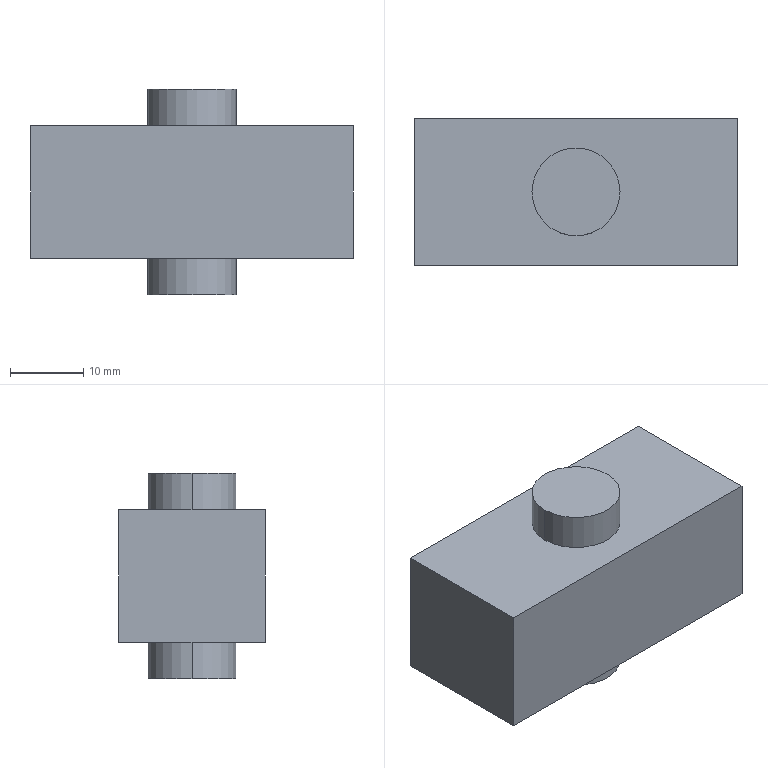Part | SolidWorks | features Extrusion 1, ICE 1 | 1 solid | 12 faces | box 44 x 20 x 28 mm | volume 16971 mm3 | plane 8 | cylinder 4 | commonest cylinder face diameters 12 x4
STEP:
#1=CARTESIAN_POINT('',(6.,0.,-14.));
#2=VERTEX_POINT('',#1);
#3=CARTESIAN_POINT('',(-6.,0.,-14.));
#4=VERTEX_POINT('',#3);
#5=CARTESIAN_POINT('',(0.,0.,-14.));
#6=DIRECTION('',(0.,0.,1.));
#7=DIRECTION('',(1.,0.,0.));
#8=AXIS2_PLACEMENT_3D('',#5,#6,#7);
#9=CIRCLE('',#8,6.);
#10=EDGE_CURVE('',#2,#4,#9,.T.);
#11=ORIENTED_EDGE('',*,*,#10,.T.);
#12=CARTESIAN_POINT('',(-6.,0.,-9.));
#13=VERTEX_POINT('',#12);
#14=CARTESIAN_POINT('',(-6.,0.,-14.));
#15=DIRECTION('',(0.,0.,1.));
#16=VECTOR('',#15,1000.);
#17=LINE('',#14,#16);
#18=EDGE_CURVE('',#4,#13,#17,.T.);
#19=ORIENTED_EDGE('',*,*,#18,.T.);
#20=CARTESIAN_POINT('',(6.,0.,-9.));
#21=VERTEX_POINT('',#20);
#22=CARTESIAN_POINT('',(0.,0.,-9.));
#23=DIRECTION('',(0.,0.,1.));
#24=DIRECTION('',(1.,0.,0.));
#25=AXIS2_PLACEMENT_3D('',#22,#23,#24);
#26=CIRCLE('',#25,6.);
#27=EDGE_CURVE('',#21,#13,#26,.T.);
#28=ORIENTED_EDGE('',*,*,#27,.F.);
#29=CARTESIAN_POINT('',(6.,0.,-14.));
#30=DIRECTION('',(0.,0.,1.));
#31=VECTOR('',#30,1000.);
#32=LINE('',#29,#31);
#33=EDGE_CURVE('',#2,#21,#32,.T.);
#34=ORIENTED_EDGE('',*,*,#33,.F.);
#35=EDGE_LOOP('',(#11,#19,#28,#34));
#36=FACE_OUTER_BOUND('',#35,.T.);
#37=CARTESIAN_POINT('',(0.,0.,-14.));
#38=DIRECTION('',(0.,0.,1.));
#39=DIRECTION('',(1.,0.,0.));
#40=AXIS2_PLACEMENT_3D('',#37,#38,#39);
#41=CYLINDRICAL_SURFACE('',#40,6.);
#42=ADVANCED_FACE('',(#36),#41,.T.);
#43=CARTESIAN_POINT('',(6.,0.,9.));
#44=VERTEX_POINT('',#43);
#45=CARTESIAN_POINT('',(-6.,0.,9.));
#46=VERTEX_POINT('',#45);
#47=CARTESIAN_POINT('',(0.,0.,9.));
#48=DIRECTION('',(0.,0.,1.));
#49=DIRECTION('',(1.,0.,0.));
#50=AXIS2_PLACEMENT_3D('',#47,#48,#49);
#51=CIRCLE('',#50,6.);
#52=EDGE_CURVE('',#44,#46,#51,.T.);
#53=ORIENTED_EDGE('',*,*,#52,.T.);
#54=CARTESIAN_POINT('',(-6.,0.,14.));
#55=VERTEX_POINT('',#54);
#56=CARTESIAN_POINT('',(-6.,0.,-14.));
#57=DIRECTION('',(0.,0.,1.));
#58=VECTOR('',#57,1000.);
#59=LINE('',#56,#58);
#60=EDGE_CURVE('',#46,#55,#59,.T.);
#61=ORIENTED_EDGE('',*,*,#60,.T.);
#62=CARTESIAN_POINT('',(6.,0.,14.));
#63=VERTEX_POINT('',#62);
#64=CARTESIAN_POINT('',(0.,0.,14.));
#65=DIRECTION('',(0.,0.,1.));
#66=DIRECTION('',(1.,0.,0.));
#67=AXIS2_PLACEMENT_3D('',#64,#65,#66);
#68=CIRCLE('',#67,6.);
#69=EDGE_CURVE('',#63,#55,#68,.T.);
#70=ORIENTED_EDGE('',*,*,#69,.F.);
#71=CARTESIAN_POINT('',(6.,0.,-14.));
#72=DIRECTION('',(0.,0.,1.));
#73=VECTOR('',#72,1000.);
#74=LINE('',#71,#73);
#75=EDGE_CURVE('',#44,#63,#74,.T.);
#76=ORIENTED_EDGE('',*,*,#75,.F.);
#77=EDGE_LOOP('',(#53,#61,#70,#76));
#78=FACE_OUTER_BOUND('',#77,.T.);
#79=CARTESIAN_POINT('',(0.,0.,-14.));
#80=DIRECTION('',(0.,0.,1.));
#81=DIRECTION('',(1.,0.,0.));
#82=AXIS2_PLACEMENT_3D('',#79,#80,#81);
#83=CYLINDRICAL_SURFACE('',#82,6.);
#84=ADVANCED_FACE('',(#78),#83,.T.);
#85=CARTESIAN_POINT('',(-22.,10.,9.));
#86=VERTEX_POINT('',#85);
#87=CARTESIAN_POINT('',(-22.,-10.,9.));
#88=VERTEX_POINT('',#87);
#89=CARTESIAN_POINT('',(-22.,10.,9.));
#90=DIRECTION('',(0.,-1.,0.));
#91=VECTOR('',#90,1000.);
#92=LINE('',#89,#91);
#93=EDGE_CURVE('',#86,#88,#92,.T.);
#94=ORIENTED_EDGE('',*,*,#93,.F.);
#95=CARTESIAN_POINT('',(-22.,10.,-9.));
#96=VERTEX_POINT('',#95);
#97=CARTESIAN_POINT('',(-22.,10.,-9.));
#98=DIRECTION('',(0.,0.,1.));
#99=VECTOR('',#98,1000.);
#100=LINE('',#97,#99);
#101=EDGE_CURVE('',#96,#86,#100,.T.);
#102=ORIENTED_EDGE('',*,*,#101,.F.);
#103=CARTESIAN_POINT('',(-22.,-10.,-9.));
#104=VERTEX_POINT('',#103);
#105=CARTESIAN_POINT('',(-22.,10.,-9.));
#106=DIRECTION('',(0.,-1.,0.));
#107=VECTOR('',#106,1000.);
#108=LINE('',#105,#107);
#109=EDGE_CURVE('',#96,#104,#108,.T.);
#110=ORIENTED_EDGE('',*,*,#109,.T.);
#111=CARTESIAN_POINT('',(-22.,-10.,-9.));
#112=DIRECTION('',(0.,0.,1.));
#113=VECTOR('',#112,1000.);
#114=LINE('',#111,#113);
#115=EDGE_CURVE('',#104,#88,#114,.T.);
#116=ORIENTED_EDGE('',*,*,#115,.T.);
#117=EDGE_LOOP('',(#94,#102,#110,#116));
#118=FACE_OUTER_BOUND('',#117,.T.);
#119=CARTESIAN_POINT('',(-22.,10.,-9.));
#120=DIRECTION('',(-1.,0.,0.));
#121=DIRECTION('',(0.,0.,1.));
#122=AXIS2_PLACEMENT_3D('',#119,#120,#121);
#123=PLANE('',#122);
#124=ADVANCED_FACE('',(#118),#123,.T.);
#125=CARTESIAN_POINT('',(22.,10.,9.));
#126=VERTEX_POINT('',#125);
#127=CARTESIAN_POINT('',(22.,10.,9.));
#128=DIRECTION('',(-1.,0.,0.));
#129=VECTOR('',#128,1000.);
#130=LINE('',#127,#129);
#131=EDGE_CURVE('',#126,#86,#130,.T.);
#132=ORIENTED_EDGE('',*,*,#131,.F.);
#133=CARTESIAN_POINT('',(22.,10.,-9.));
#134=VERTEX_POINT('',#133);
#135=CARTESIAN_POINT('',(22.,10.,-9.));
#136=DIRECTION('',(0.,0.,1.));
#137=VECTOR('',#136,1000.);
#138=LINE('',#135,#137);
#139=EDGE_CURVE('',#134,#126,#138,.T.);
#140=ORIENTED_EDGE('',*,*,#139,.F.);
#141=CARTESIAN_POINT('',(22.,10.,-9.));
#142=DIRECTION('',(-1.,0.,0.));
#143=VECTOR('',#142,1000.);
#144=LINE('',#141,#143);
#145=EDGE_CURVE('',#134,#96,#144,.T.);
#146=ORIENTED_EDGE('',*,*,#145,.T.);
#147=ORIENTED_EDGE('',*,*,#101,.T.);
#148=EDGE_LOOP('',(#132,#140,#146,#147));
#149=FACE_OUTER_BOUND('',#148,.T.);
#150=CARTESIAN_POINT('',(22.,10.,-9.));
#151=DIRECTION('',(0.,1.,0.));
#152=DIRECTION('',(0.,0.,1.));
#153=AXIS2_PLACEMENT_3D('',#150,#151,#152);
#154=PLANE('',#153);
#155=ADVANCED_FACE('',(#149),#154,.T.);
#156=CARTESIAN_POINT('',(22.,-10.,9.));
#157=VERTEX_POINT('',#156);
#158=CARTESIAN_POINT('',(22.,-10.,9.));
#159=DIRECTION('',(0.,1.,0.));
#160=VECTOR('',#159,1000.);
#161=LINE('',#158,#160);
#162=EDGE_CURVE('',#157,#126,#161,.T.);
#163=ORIENTED_EDGE('',*,*,#162,.F.);
#164=CARTESIAN_POINT('',(22.,-10.,-9.));
#165=VERTEX_POINT('',#164);
#166=CARTESIAN_POINT('',(22.,-10.,-9.));
#167=DIRECTION('',(0.,0.,1.));
#168=VECTOR('',#167,1000.);
#169=LINE('',#166,#168);
#170=EDGE_CURVE('',#165,#157,#169,.T.);
#171=ORIENTED_EDGE('',*,*,#170,.F.);
#172=CARTESIAN_POINT('',(22.,-10.,-9.));
#173=DIRECTION('',(0.,1.,0.));
#174=VECTOR('',#173,1000.);
#175=LINE('',#172,#174);
#176=EDGE_CURVE('',#165,#134,#175,.T.);
#177=ORIENTED_EDGE('',*,*,#176,.T.);
#178=ORIENTED_EDGE('',*,*,#139,.T.);
#179=EDGE_LOOP('',(#163,#171,#177,#178));
#180=FACE_OUTER_BOUND('',#179,.T.);
#181=CARTESIAN_POINT('',(22.,-10.,-9.));
#182=DIRECTION('',(1.,0.,0.));
#183=DIRECTION('',(0.,0.,-1.));
#184=AXIS2_PLACEMENT_3D('',#181,#182,#183);
#185=PLANE('',#184);
#186=ADVANCED_FACE('',(#180),#185,.T.);
#187=CARTESIAN_POINT('',(-22.,-10.,9.));
#188=DIRECTION('',(1.,0.,0.));
#189=VECTOR('',#188,1000.);
#190=LINE('',#187,#189);
#191=EDGE_CURVE('',#88,#157,#190,.T.);
#192=ORIENTED_EDGE('',*,*,#191,.F.);
#193=ORIENTED_EDGE('',*,*,#115,.F.);
#194=CARTESIAN_POINT('',(-22.,-10.,-9.));
#195=DIRECTION('',(1.,0.,0.));
#196=VECTOR('',#195,1000.);
#197=LINE('',#194,#196);
#198=EDGE_CURVE('',#104,#165,#197,.T.);
#199=ORIENTED_EDGE('',*,*,#198,.T.);
#200=ORIENTED_EDGE('',*,*,#170,.T.);
#201=EDGE_LOOP('',(#192,#193,#199,#200));
#202=FACE_OUTER_BOUND('',#201,.T.);
#203=CARTESIAN_POINT('',(-22.,-10.,-9.));
#204=DIRECTION('',(0.,-1.,0.));
#205=DIRECTION('',(0.,0.,-1.));
#206=AXIS2_PLACEMENT_3D('',#203,#204,#205);
#207=PLANE('',#206);
#208=ADVANCED_FACE('',(#202),#207,.T.);
#209=ORIENTED_EDGE('',*,*,#27,.T.);
#210=CARTESIAN_POINT('',(0.,0.,-9.));
#211=DIRECTION('',(0.,0.,1.));
#212=DIRECTION('',(1.,0.,0.));
#213=AXIS2_PLACEMENT_3D('',#210,#211,#212);
#214=CIRCLE('',#213,6.);
#215=EDGE_CURVE('',#13,#21,#214,.T.);
#216=ORIENTED_EDGE('',*,*,#215,.T.);
#217=EDGE_LOOP('',(#209,#216));
#218=FACE_BOUND('',#217,.T.);
#219=ORIENTED_EDGE('',*,*,#109,.F.);
#220=ORIENTED_EDGE('',*,*,#145,.F.);
#221=ORIENTED_EDGE('',*,*,#176,.F.);
#222=ORIENTED_EDGE('',*,*,#198,.F.);
#223=EDGE_LOOP('',(#219,#220,#221,#222));
#224=FACE_OUTER_BOUND('',#223,.T.);
#225=CARTESIAN_POINT('',(0.,0.,-9.));
#226=DIRECTION('',(0.,0.,1.));
#227=DIRECTION('',(1.,0.,0.));
#228=AXIS2_PLACEMENT_3D('',#225,#226,#227);
#229=PLANE('',#228);
#230=ADVANCED_FACE('',(#218,#224),#229,.F.);
#231=ORIENTED_EDGE('',*,*,#52,.F.);
#232=CARTESIAN_POINT('',(0.,0.,9.));
#233=DIRECTION('',(0.,0.,1.));
#234=DIRECTION('',(1.,0.,0.));
#235=AXIS2_PLACEMENT_3D('',#232,#233,#234);
#236=CIRCLE('',#235,6.);
#237=EDGE_CURVE('',#46,#44,#236,.T.);
#238=ORIENTED_EDGE('',*,*,#237,.F.);
#239=EDGE_LOOP('',(#231,#238));
#240=FACE_BOUND('',#239,.T.);
#241=ORIENTED_EDGE('',*,*,#93,.T.);
#242=ORIENTED_EDGE('',*,*,#191,.T.);
#243=ORIENTED_EDGE('',*,*,#162,.T.);
#244=ORIENTED_EDGE('',*,*,#131,.T.);
#245=EDGE_LOOP('',(#241,#242,#243,#244));
#246=FACE_OUTER_BOUND('',#245,.T.);
#247=CARTESIAN_POINT('',(0.,0.,9.));
#248=DIRECTION('',(0.,0.,1.));
#249=DIRECTION('',(1.,0.,0.));
#250=AXIS2_PLACEMENT_3D('',#247,#248,#249);
#251=PLANE('',#250);
#252=ADVANCED_FACE('',(#240,#246),#251,.T.);
#253=ORIENTED_EDGE('',*,*,#69,.T.);
#254=CARTESIAN_POINT('',(0.,0.,14.));
#255=DIRECTION('',(0.,0.,1.));
#256=DIRECTION('',(1.,0.,0.));
#257=AXIS2_PLACEMENT_3D('',#254,#255,#256);
#258=CIRCLE('',#257,6.);
#259=EDGE_CURVE('',#55,#63,#258,.T.);
#260=ORIENTED_EDGE('',*,*,#259,.T.);
#261=EDGE_LOOP('',(#253,#260));
#262=FACE_OUTER_BOUND('',#261,.T.);
#263=CARTESIAN_POINT('',(0.,0.,14.));
#264=DIRECTION('',(0.,0.,1.));
#265=DIRECTION('',(1.,0.,0.));
#266=AXIS2_PLACEMENT_3D('',#263,#264,#265);
#267=PLANE('',#266);
#268=ADVANCED_FACE('',(#262),#267,.T.);
#269=ORIENTED_EDGE('',*,*,#60,.F.);
#270=ORIENTED_EDGE('',*,*,#237,.T.);
#271=ORIENTED_EDGE('',*,*,#75,.T.);
#272=ORIENTED_EDGE('',*,*,#259,.F.);
#273=EDGE_LOOP('',(#269,#270,#271,#272));
#274=FACE_OUTER_BOUND('',#273,.T.);
#275=CARTESIAN_POINT('',(0.,0.,-14.));
#276=DIRECTION('',(0.,0.,1.));
#277=DIRECTION('',(1.,0.,0.));
#278=AXIS2_PLACEMENT_3D('',#275,#276,#277);
#279=CYLINDRICAL_SURFACE('',#278,6.);
#280=ADVANCED_FACE('',(#274),#279,.T.);
#281=ORIENTED_EDGE('',*,*,#18,.F.);
#282=CARTESIAN_POINT('',(0.,0.,-14.));
#283=DIRECTION('',(0.,0.,1.));
#284=DIRECTION('',(1.,0.,0.));
#285=AXIS2_PLACEMENT_3D('',#282,#283,#284);
#286=CIRCLE('',#285,6.);
#287=EDGE_CURVE('',#4,#2,#286,.T.);
#288=ORIENTED_EDGE('',*,*,#287,.T.);
#289=ORIENTED_EDGE('',*,*,#33,.T.);
#290=ORIENTED_EDGE('',*,*,#215,.F.);
#291=EDGE_LOOP('',(#281,#288,#289,#290));
#292=FACE_OUTER_BOUND('',#291,.T.);
#293=CARTESIAN_POINT('',(0.,0.,-14.));
#294=DIRECTION('',(0.,0.,1.));
#295=DIRECTION('',(1.,0.,0.));
#296=AXIS2_PLACEMENT_3D('',#293,#294,#295);
#297=CYLINDRICAL_SURFACE('',#296,6.);
#298=ADVANCED_FACE('',(#292),#297,.T.);
#299=ORIENTED_EDGE('',*,*,#10,.F.);
#300=ORIENTED_EDGE('',*,*,#287,.F.);
#301=EDGE_LOOP('',(#299,#300));
#302=FACE_OUTER_BOUND('',#301,.T.);
#303=CARTESIAN_POINT('',(0.,0.,-14.));
#304=DIRECTION('',(0.,0.,1.));
#305=DIRECTION('',(1.,0.,0.));
#306=AXIS2_PLACEMENT_3D('',#303,#304,#305);
#307=PLANE('',#306);
#308=ADVANCED_FACE('',(#302),#307,.F.);
#309=CLOSED_SHELL('',(#42,#84,#124,#155,#186,#208,#230,#252,#268,#280,#298,#308));
#310=MANIFOLD_SOLID_BREP('',#309);
#311=CARTESIAN_POINT('',(0.,0.,0.));
#312=DIRECTION('',(0.,0.,1.));
#313=DIRECTION('',(1.,0.,0.));
#314=AXIS2_PLACEMENT_3D('',#311,#312,#313);
#315=(LENGTH_UNIT()NAMED_UNIT(*)SI_UNIT(.MILLI.,.METRE.));
#316=UNCERTAINTY_MEASURE_WITH_UNIT(LENGTH_MEASURE(0.00001),#315,'','');
#317=(NAMED_UNIT(*)PLANE_ANGLE_UNIT()SI_UNIT($,.RADIAN.));
#318=(NAMED_UNIT(*)SI_UNIT($,.STERADIAN.)SOLID_ANGLE_UNIT());
#319=(GEOMETRIC_REPRESENTATION_CONTEXT(3)GLOBAL_UNCERTAINTY_ASSIGNED_CONTEXT((#316))GLOBAL_UNIT_ASSIGNED_CONTEXT((#315,#317,#318))REPRESENTATION_CONTEXT('',''));
#320=ADVANCED_BREP_SHAPE_REPRESENTATION('',(#310,#314),#319);